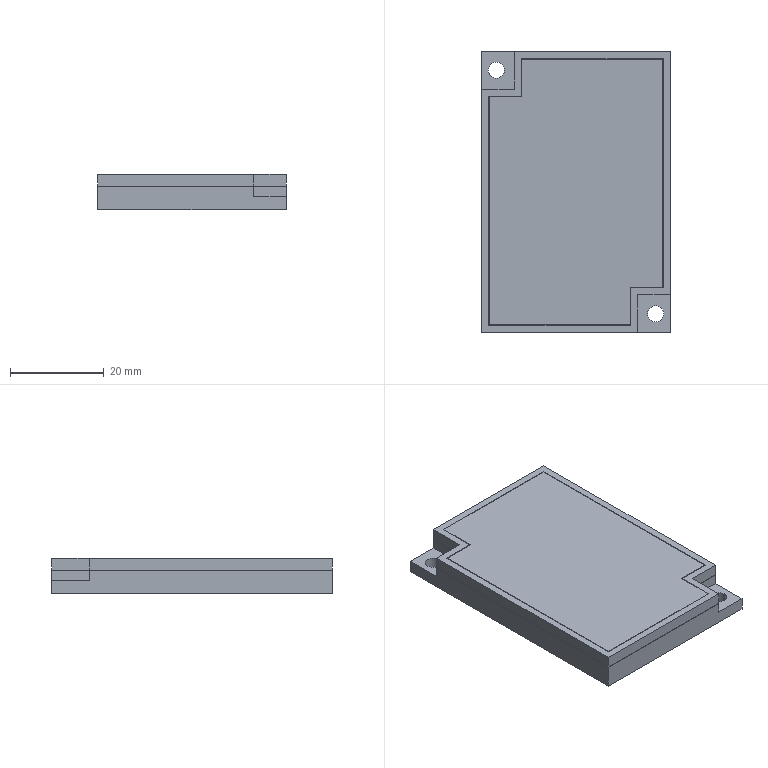Part | STEP file | E39-R1_PART1 | 1 solid | 52 faces | box 40.3 x 59.9 x 7.5 mm | volume 17477 mm3 | plane 48 | cylinder 4 | commonest cylinder face diameters 3.5 x4